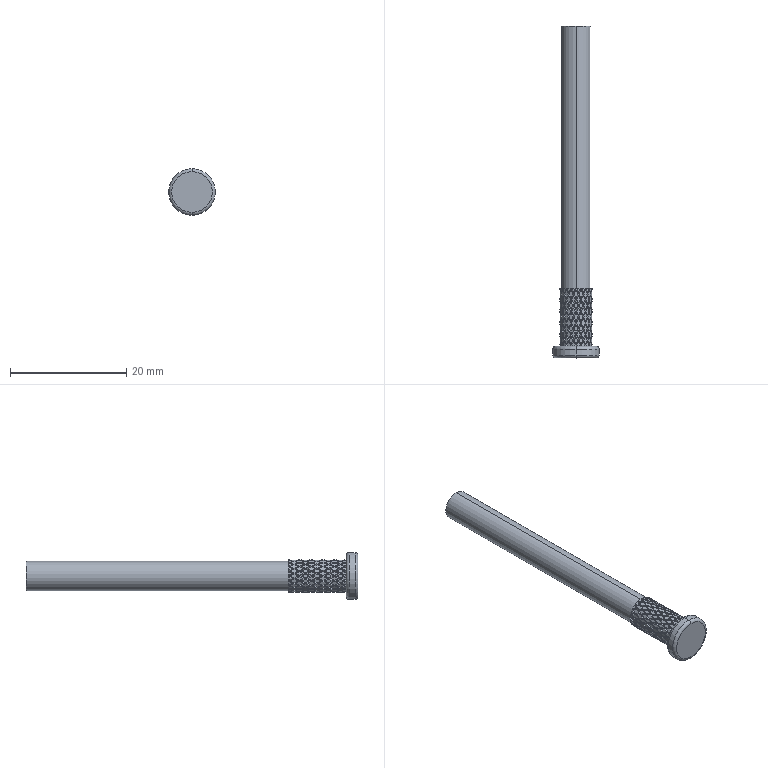Part | STEP file | 1 solid | 1162 faces | box 8 x 57 x 8 mm | volume 1212 mm3 | spline 900 | cylinder 230 | plane 28 | torus 4 | commonest cylinder face diameters 5.5 x226 5 x2 8 x2